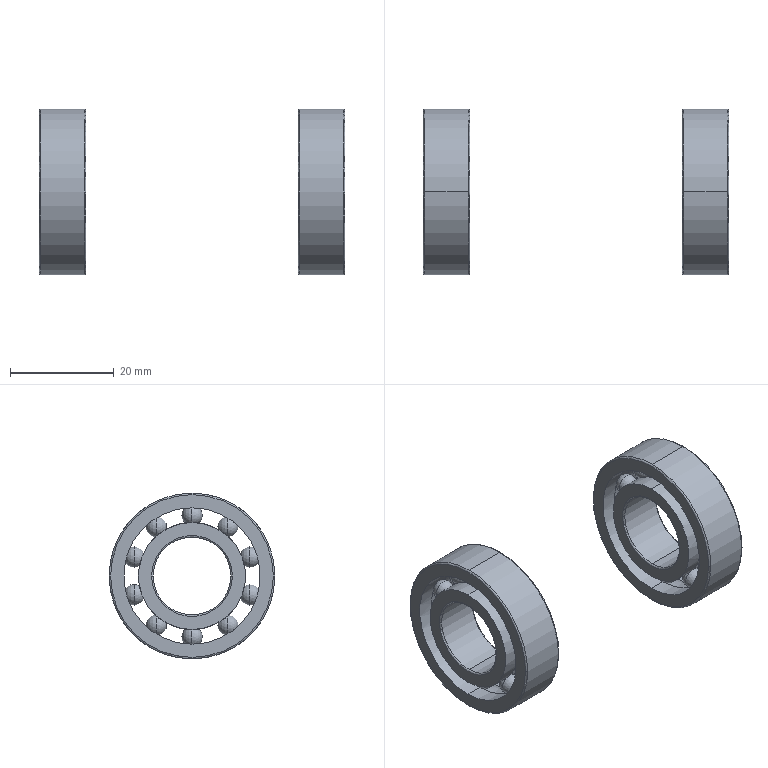Part | NX | 2 solids | 154 faces | box 59 x 32 x 32 mm | volume 7930 mm3 | torus 82 | sphere 40 | cylinder 24 | plane 8 | commonest cylinder face diameters 20.667 x8 26.333 x8 15 x4 32 x4